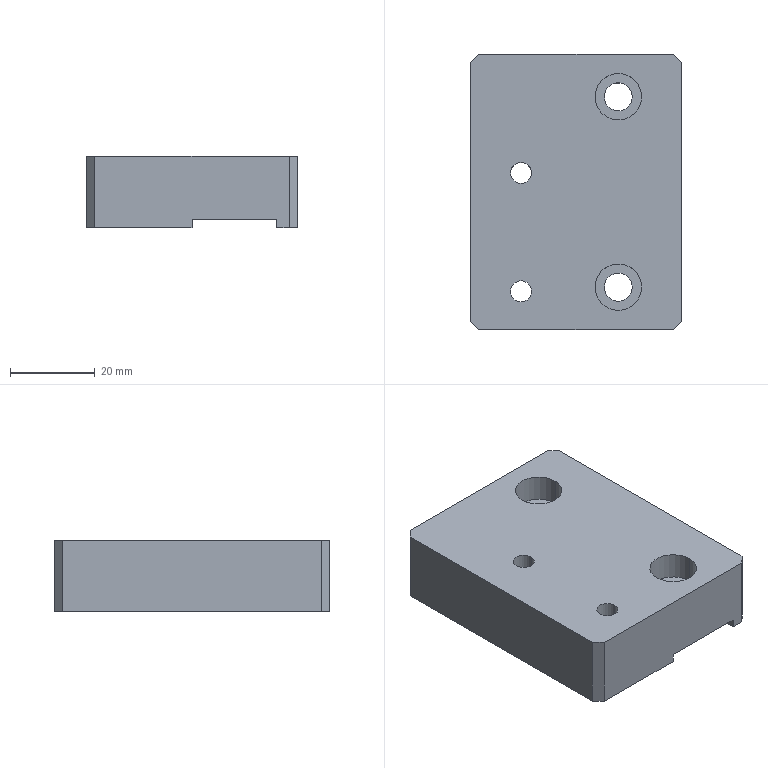Part | SolidWorks | features HoleWzd 2, Chamfer 1, Extrusion 1, ICE 1 | 1 solid | 28 faces | box 50 x 65 x 17 mm | volume 50042 mm3 | plane 16 | cylinder 12 | commonest cylinder face diameters 5 x4 6.6 x4 11 x4
STEP:
#1=CARTESIAN_POINT('',(29.5,-10.,10.6));
#2=VERTEX_POINT('',#1);
#3=CARTESIAN_POINT('',(40.5,-10.,10.6));
#4=VERTEX_POINT('',#3);
#5=CARTESIAN_POINT('',(35.,-10.,10.6));
#6=DIRECTION('',(0.,0.,1.));
#7=DIRECTION('',(1.,0.,0.));
#8=AXIS2_PLACEMENT_3D('',#5,#6,#7);
#9=CIRCLE('',#8,5.5);
#10=EDGE_CURVE('',#2,#4,#9,.T.);
#11=ORIENTED_EDGE('',*,*,#10,.F.);
#12=CARTESIAN_POINT('',(29.5,-10.,17.));
#13=VERTEX_POINT('',#12);
#14=CARTESIAN_POINT('',(29.5,-10.,17.));
#15=DIRECTION('',(0.,0.,1.));
#16=VECTOR('',#15,1000.);
#17=LINE('',#14,#16);
#18=EDGE_CURVE('',#2,#13,#17,.T.);
#19=ORIENTED_EDGE('',*,*,#18,.T.);
#20=CARTESIAN_POINT('',(40.5,-10.,17.));
#21=VERTEX_POINT('',#20);
#22=CARTESIAN_POINT('',(35.,-10.,17.));
#23=DIRECTION('',(0.,0.,1.));
#24=DIRECTION('',(1.,0.,0.));
#25=AXIS2_PLACEMENT_3D('',#22,#23,#24);
#26=CIRCLE('',#25,5.5);
#27=EDGE_CURVE('',#13,#21,#26,.T.);
#28=ORIENTED_EDGE('',*,*,#27,.T.);
#29=CARTESIAN_POINT('',(40.5,-10.,17.));
#30=DIRECTION('',(0.,0.,1.));
#31=VECTOR('',#30,1000.);
#32=LINE('',#29,#31);
#33=EDGE_CURVE('',#4,#21,#32,.T.);
#34=ORIENTED_EDGE('',*,*,#33,.F.);
#35=EDGE_LOOP('',(#11,#19,#28,#34));
#36=FACE_OUTER_BOUND('',#35,.T.);
#37=CARTESIAN_POINT('',(35.,-10.,17.));
#38=DIRECTION('',(0.,0.,1.));
#39=DIRECTION('',(1.,0.,0.));
#40=AXIS2_PLACEMENT_3D('',#37,#38,#39);
#41=CYLINDRICAL_SURFACE('',#40,5.5);
#42=ADVANCED_FACE('',(#36),#41,.F.);
#43=CARTESIAN_POINT('',(31.7,-10.,2.));
#44=VERTEX_POINT('',#43);
#45=CARTESIAN_POINT('',(38.3,-10.,2.));
#46=VERTEX_POINT('',#45);
#47=CARTESIAN_POINT('',(35.,-10.,2.));
#48=DIRECTION('',(0.,0.,1.));
#49=DIRECTION('',(1.,0.,0.));
#50=AXIS2_PLACEMENT_3D('',#47,#48,#49);
#51=CIRCLE('',#50,3.3);
#52=EDGE_CURVE('',#44,#46,#51,.T.);
#53=ORIENTED_EDGE('',*,*,#52,.F.);
#54=CARTESIAN_POINT('',(31.7,-10.,10.6));
#55=VERTEX_POINT('',#54);
#56=CARTESIAN_POINT('',(31.7,-10.,17.));
#57=DIRECTION('',(0.,0.,1.));
#58=VECTOR('',#57,1000.);
#59=LINE('',#56,#58);
#60=EDGE_CURVE('',#44,#55,#59,.T.);
#61=ORIENTED_EDGE('',*,*,#60,.T.);
#62=CARTESIAN_POINT('',(38.3,-10.,10.6));
#63=VERTEX_POINT('',#62);
#64=CARTESIAN_POINT('',(35.,-10.,10.6));
#65=DIRECTION('',(0.,0.,1.));
#66=DIRECTION('',(1.,0.,0.));
#67=AXIS2_PLACEMENT_3D('',#64,#65,#66);
#68=CIRCLE('',#67,3.3);
#69=EDGE_CURVE('',#55,#63,#68,.T.);
#70=ORIENTED_EDGE('',*,*,#69,.T.);
#71=CARTESIAN_POINT('',(38.3,-10.,17.));
#72=DIRECTION('',(0.,0.,1.));
#73=VECTOR('',#72,1000.);
#74=LINE('',#71,#73);
#75=EDGE_CURVE('',#46,#63,#74,.T.);
#76=ORIENTED_EDGE('',*,*,#75,.F.);
#77=EDGE_LOOP('',(#53,#61,#70,#76));
#78=FACE_OUTER_BOUND('',#77,.T.);
#79=CARTESIAN_POINT('',(35.,-10.,17.));
#80=DIRECTION('',(0.,0.,1.));
#81=DIRECTION('',(1.,0.,0.));
#82=AXIS2_PLACEMENT_3D('',#79,#80,#81);
#83=CYLINDRICAL_SURFACE('',#82,3.3);
#84=ADVANCED_FACE('',(#78),#83,.F.);
#85=CARTESIAN_POINT('',(29.5,-55.,10.6));
#86=VERTEX_POINT('',#85);
#87=CARTESIAN_POINT('',(40.5,-55.,10.6));
#88=VERTEX_POINT('',#87);
#89=CARTESIAN_POINT('',(35.,-55.,10.6));
#90=DIRECTION('',(0.,0.,1.));
#91=DIRECTION('',(1.,0.,0.));
#92=AXIS2_PLACEMENT_3D('',#89,#90,#91);
#93=CIRCLE('',#92,5.5);
#94=EDGE_CURVE('',#86,#88,#93,.T.);
#95=ORIENTED_EDGE('',*,*,#94,.F.);
#96=CARTESIAN_POINT('',(29.5,-55.,17.));
#97=VERTEX_POINT('',#96);
#98=CARTESIAN_POINT('',(29.5,-55.,17.));
#99=DIRECTION('',(0.,0.,1.));
#100=VECTOR('',#99,1000.);
#101=LINE('',#98,#100);
#102=EDGE_CURVE('',#86,#97,#101,.T.);
#103=ORIENTED_EDGE('',*,*,#102,.T.);
#104=CARTESIAN_POINT('',(40.5,-55.,17.));
#105=VERTEX_POINT('',#104);
#106=CARTESIAN_POINT('',(35.,-55.,17.));
#107=DIRECTION('',(0.,0.,1.));
#108=DIRECTION('',(1.,0.,0.));
#109=AXIS2_PLACEMENT_3D('',#106,#107,#108);
#110=CIRCLE('',#109,5.5);
#111=EDGE_CURVE('',#97,#105,#110,.T.);
#112=ORIENTED_EDGE('',*,*,#111,.T.);
#113=CARTESIAN_POINT('',(40.5,-55.,17.));
#114=DIRECTION('',(0.,0.,1.));
#115=VECTOR('',#114,1000.);
#116=LINE('',#113,#115);
#117=EDGE_CURVE('',#88,#105,#116,.T.);
#118=ORIENTED_EDGE('',*,*,#117,.F.);
#119=EDGE_LOOP('',(#95,#103,#112,#118));
#120=FACE_OUTER_BOUND('',#119,.T.);
#121=CARTESIAN_POINT('',(35.,-55.,17.));
#122=DIRECTION('',(0.,0.,1.));
#123=DIRECTION('',(1.,0.,0.));
#124=AXIS2_PLACEMENT_3D('',#121,#122,#123);
#125=CYLINDRICAL_SURFACE('',#124,5.5);
#126=ADVANCED_FACE('',(#120),#125,.F.);
#127=CARTESIAN_POINT('',(31.7,-55.,2.));
#128=VERTEX_POINT('',#127);
#129=CARTESIAN_POINT('',(38.3,-55.,2.));
#130=VERTEX_POINT('',#129);
#131=CARTESIAN_POINT('',(35.,-55.,2.));
#132=DIRECTION('',(0.,0.,1.));
#133=DIRECTION('',(1.,0.,0.));
#134=AXIS2_PLACEMENT_3D('',#131,#132,#133);
#135=CIRCLE('',#134,3.3);
#136=EDGE_CURVE('',#128,#130,#135,.T.);
#137=ORIENTED_EDGE('',*,*,#136,.F.);
#138=CARTESIAN_POINT('',(31.7,-55.,10.6));
#139=VERTEX_POINT('',#138);
#140=CARTESIAN_POINT('',(31.7,-55.,17.));
#141=DIRECTION('',(0.,0.,1.));
#142=VECTOR('',#141,1000.);
#143=LINE('',#140,#142);
#144=EDGE_CURVE('',#128,#139,#143,.T.);
#145=ORIENTED_EDGE('',*,*,#144,.T.);
#146=CARTESIAN_POINT('',(38.3,-55.,10.6));
#147=VERTEX_POINT('',#146);
#148=CARTESIAN_POINT('',(35.,-55.,10.6));
#149=DIRECTION('',(0.,0.,1.));
#150=DIRECTION('',(1.,0.,0.));
#151=AXIS2_PLACEMENT_3D('',#148,#149,#150);
#152=CIRCLE('',#151,3.3);
#153=EDGE_CURVE('',#139,#147,#152,.T.);
#154=ORIENTED_EDGE('',*,*,#153,.T.);
#155=CARTESIAN_POINT('',(38.3,-55.,17.));
#156=DIRECTION('',(0.,0.,1.));
#157=VECTOR('',#156,1000.);
#158=LINE('',#155,#157);
#159=EDGE_CURVE('',#130,#147,#158,.T.);
#160=ORIENTED_EDGE('',*,*,#159,.F.);
#161=EDGE_LOOP('',(#137,#145,#154,#160));
#162=FACE_OUTER_BOUND('',#161,.T.);
#163=CARTESIAN_POINT('',(35.,-55.,17.));
#164=DIRECTION('',(0.,0.,1.));
#165=DIRECTION('',(1.,0.,0.));
#166=AXIS2_PLACEMENT_3D('',#163,#164,#165);
#167=CYLINDRICAL_SURFACE('',#166,3.3);
#168=ADVANCED_FACE('',(#162),#167,.F.);
#169=CARTESIAN_POINT('',(9.5,-28.,0.));
#170=VERTEX_POINT('',#169);
#171=CARTESIAN_POINT('',(14.5,-28.,0.));
#172=VERTEX_POINT('',#171);
#173=CARTESIAN_POINT('',(12.,-28.,0.));
#174=DIRECTION('',(0.,0.,1.));
#175=DIRECTION('',(1.,0.,0.));
#176=AXIS2_PLACEMENT_3D('',#173,#174,#175);
#177=CIRCLE('',#176,2.5);
#178=EDGE_CURVE('',#170,#172,#177,.T.);
#179=ORIENTED_EDGE('',*,*,#178,.F.);
#180=CARTESIAN_POINT('',(9.5,-28.,17.));
#181=VERTEX_POINT('',#180);
#182=CARTESIAN_POINT('',(9.5,-28.,17.));
#183=DIRECTION('',(0.,0.,1.));
#184=VECTOR('',#183,1000.);
#185=LINE('',#182,#184);
#186=EDGE_CURVE('',#170,#181,#185,.T.);
#187=ORIENTED_EDGE('',*,*,#186,.T.);
#188=CARTESIAN_POINT('',(14.5,-28.,17.));
#189=VERTEX_POINT('',#188);
#190=CARTESIAN_POINT('',(12.,-28.,17.));
#191=DIRECTION('',(0.,0.,1.));
#192=DIRECTION('',(1.,0.,0.));
#193=AXIS2_PLACEMENT_3D('',#190,#191,#192);
#194=CIRCLE('',#193,2.5);
#195=EDGE_CURVE('',#181,#189,#194,.T.);
#196=ORIENTED_EDGE('',*,*,#195,.T.);
#197=CARTESIAN_POINT('',(14.5,-28.,17.));
#198=DIRECTION('',(0.,0.,1.));
#199=VECTOR('',#198,1000.);
#200=LINE('',#197,#199);
#201=EDGE_CURVE('',#172,#189,#200,.T.);
#202=ORIENTED_EDGE('',*,*,#201,.F.);
#203=EDGE_LOOP('',(#179,#187,#196,#202));
#204=FACE_OUTER_BOUND('',#203,.T.);
#205=CARTESIAN_POINT('',(12.,-28.,17.));
#206=DIRECTION('',(0.,0.,1.));
#207=DIRECTION('',(1.,0.,0.));
#208=AXIS2_PLACEMENT_3D('',#205,#206,#207);
#209=CYLINDRICAL_SURFACE('',#208,2.5);
#210=ADVANCED_FACE('',(#204),#209,.F.);
#211=CARTESIAN_POINT('',(9.5,-56.,0.));
#212=VERTEX_POINT('',#211);
#213=CARTESIAN_POINT('',(14.5,-56.,0.));
#214=VERTEX_POINT('',#213);
#215=CARTESIAN_POINT('',(12.,-56.,0.));
#216=DIRECTION('',(0.,0.,1.));
#217=DIRECTION('',(1.,0.,0.));
#218=AXIS2_PLACEMENT_3D('',#215,#216,#217);
#219=CIRCLE('',#218,2.5);
#220=EDGE_CURVE('',#212,#214,#219,.T.);
#221=ORIENTED_EDGE('',*,*,#220,.F.);
#222=CARTESIAN_POINT('',(9.5,-56.,17.));
#223=VERTEX_POINT('',#222);
#224=CARTESIAN_POINT('',(9.5,-56.,17.));
#225=DIRECTION('',(0.,0.,1.));
#226=VECTOR('',#225,1000.);
#227=LINE('',#224,#226);
#228=EDGE_CURVE('',#212,#223,#227,.T.);
#229=ORIENTED_EDGE('',*,*,#228,.T.);
#230=CARTESIAN_POINT('',(14.5,-56.,17.));
#231=VERTEX_POINT('',#230);
#232=CARTESIAN_POINT('',(12.,-56.,17.));
#233=DIRECTION('',(0.,0.,1.));
#234=DIRECTION('',(1.,0.,0.));
#235=AXIS2_PLACEMENT_3D('',#232,#233,#234);
#236=CIRCLE('',#235,2.5);
#237=EDGE_CURVE('',#223,#231,#236,.T.);
#238=ORIENTED_EDGE('',*,*,#237,.T.);
#239=CARTESIAN_POINT('',(14.5,-56.,17.));
#240=DIRECTION('',(0.,0.,1.));
#241=VECTOR('',#240,1000.);
#242=LINE('',#239,#241);
#243=EDGE_CURVE('',#214,#231,#242,.T.);
#244=ORIENTED_EDGE('',*,*,#243,.F.);
#245=EDGE_LOOP('',(#221,#229,#238,#244));
#246=FACE_OUTER_BOUND('',#245,.T.);
#247=CARTESIAN_POINT('',(12.,-56.,17.));
#248=DIRECTION('',(0.,0.,1.));
#249=DIRECTION('',(1.,0.,0.));
#250=AXIS2_PLACEMENT_3D('',#247,#248,#249);
#251=CYLINDRICAL_SURFACE('',#250,2.5);
#252=ADVANCED_FACE('',(#246),#251,.F.);
#253=CARTESIAN_POINT('',(50.,-63.,0.));
#254=VERTEX_POINT('',#253);
#255=CARTESIAN_POINT('',(50.,-2.,0.));
#256=VERTEX_POINT('',#255);
#257=CARTESIAN_POINT('',(50.,0.,0.));
#258=DIRECTION('',(0.,1.,0.));
#259=VECTOR('',#258,1000.);
#260=LINE('',#257,#259);
#261=EDGE_CURVE('',#254,#256,#260,.T.);
#262=ORIENTED_EDGE('',*,*,#261,.F.);
#263=CARTESIAN_POINT('',(48.,-65.,0.));
#264=VERTEX_POINT('',#263);
#265=CARTESIAN_POINT('',(50.,-63.,0.));
#266=DIRECTION('',(-0.7071,-0.7071,0.));
#267=VECTOR('',#266,1000.);
#268=LINE('',#265,#267);
#269=EDGE_CURVE('',#254,#264,#268,.T.);
#270=ORIENTED_EDGE('',*,*,#269,.T.);
#271=CARTESIAN_POINT('',(45.,-65.,0.));
#272=VERTEX_POINT('',#271);
#273=CARTESIAN_POINT('',(0.,-65.,0.));
#274=DIRECTION('',(1.,0.,0.));
#275=VECTOR('',#274,1000.);
#276=LINE('',#273,#275);
#277=EDGE_CURVE('',#272,#264,#276,.T.);
#278=ORIENTED_EDGE('',*,*,#277,.F.);
#279=CARTESIAN_POINT('',(45.,0.,0.));
#280=VERTEX_POINT('',#279);
#281=CARTESIAN_POINT('',(45.,0.,0.));
#282=DIRECTION('',(0.,-1.,0.));
#283=VECTOR('',#282,1000.);
#284=LINE('',#281,#283);
#285=EDGE_CURVE('',#280,#272,#284,.T.);
#286=ORIENTED_EDGE('',*,*,#285,.F.);
#287=CARTESIAN_POINT('',(48.,0.,0.));
#288=VERTEX_POINT('',#287);
#289=CARTESIAN_POINT('',(0.,0.,0.));
#290=DIRECTION('',(-1.,0.,0.));
#291=VECTOR('',#290,1000.);
#292=LINE('',#289,#291);
#293=EDGE_CURVE('',#288,#280,#292,.T.);
#294=ORIENTED_EDGE('',*,*,#293,.F.);
#295=CARTESIAN_POINT('',(48.,0.,0.));
#296=DIRECTION('',(0.7071,-0.7071,0.));
#297=VECTOR('',#296,1000.);
#298=LINE('',#295,#297);
#299=EDGE_CURVE('',#288,#256,#298,.T.);
#300=ORIENTED_EDGE('',*,*,#299,.T.);
#301=EDGE_LOOP('',(#262,#270,#278,#286,#294,#300));
#302=FACE_OUTER_BOUND('',#301,.T.);
#303=CARTESIAN_POINT('',(0.,0.,0.));
#304=DIRECTION('',(0.,0.,1.));
#305=DIRECTION('',(1.,0.,0.));
#306=AXIS2_PLACEMENT_3D('',#303,#304,#305);
#307=PLANE('',#306);
#308=ADVANCED_FACE('',(#302),#307,.F.);
#309=CARTESIAN_POINT('',(0.,-2.,17.));
#310=VERTEX_POINT('',#309);
#311=CARTESIAN_POINT('',(0.,-63.,17.));
#312=VERTEX_POINT('',#311);
#313=CARTESIAN_POINT('',(0.,0.,17.));
#314=DIRECTION('',(0.,-1.,0.));
#315=VECTOR('',#314,1000.);
#316=LINE('',#313,#315);
#317=EDGE_CURVE('',#310,#312,#316,.T.);
#318=ORIENTED_EDGE('',*,*,#317,.F.);
#319=CARTESIAN_POINT('',(0.,-2.,0.));
#320=VERTEX_POINT('',#319);
#321=CARTESIAN_POINT('',(0.,-2.,17.));
#322=DIRECTION('',(0.,0.,-1.));
#323=VECTOR('',#322,1000.);
#324=LINE('',#321,#323);
#325=EDGE_CURVE('',#310,#320,#324,.T.);
#326=ORIENTED_EDGE('',*,*,#325,.T.);
#327=CARTESIAN_POINT('',(0.,-63.,0.));
#328=VERTEX_POINT('',#327);
#329=CARTESIAN_POINT('',(0.,0.,0.));
#330=DIRECTION('',(0.,-1.,0.));
#331=VECTOR('',#330,1000.);
#332=LINE('',#329,#331);
#333=EDGE_CURVE('',#320,#328,#332,.T.);
#334=ORIENTED_EDGE('',*,*,#333,.T.);
#335=CARTESIAN_POINT('',(0.,-63.,17.));
#336=DIRECTION('',(0.,0.,1.));
#337=VECTOR('',#336,1000.);
#338=LINE('',#335,#337);
#339=EDGE_CURVE('',#328,#312,#338,.T.);
#340=ORIENTED_EDGE('',*,*,#339,.T.);
#341=EDGE_LOOP('',(#318,#326,#334,#340));
#342=FACE_OUTER_BOUND('',#341,.T.);
#343=CARTESIAN_POINT('',(0.,0.,17.));
#344=DIRECTION('',(1.,0.,0.));
#345=DIRECTION('',(0.,0.,-1.));
#346=AXIS2_PLACEMENT_3D('',#343,#344,#345);
#347=PLANE('',#346);
#348=ADVANCED_FACE('',(#342),#347,.F.);
#349=ORIENTED_EDGE('',*,*,#277,.T.);
#350=CARTESIAN_POINT('',(48.,-65.,17.));
#351=VERTEX_POINT('',#350);
#352=CARTESIAN_POINT('',(48.,-65.,17.));
#353=DIRECTION('',(0.,0.,1.));
#354=VECTOR('',#353,1000.);
#355=LINE('',#352,#354);
#356=EDGE_CURVE('',#264,#351,#355,.T.);
#357=ORIENTED_EDGE('',*,*,#356,.T.);
#358=CARTESIAN_POINT('',(2.,-65.,17.));
#359=VERTEX_POINT('',#358);
#360=CARTESIAN_POINT('',(0.,-65.,17.));
#361=DIRECTION('',(1.,0.,0.));
#362=VECTOR('',#361,1000.);
#363=LINE('',#360,#362);
#364=EDGE_CURVE('',#359,#351,#363,.T.);
#365=ORIENTED_EDGE('',*,*,#364,.F.);
#366=CARTESIAN_POINT('',(2.,-65.,0.));
#367=VERTEX_POINT('',#366);
#368=CARTESIAN_POINT('',(2.,-65.,17.));
#369=DIRECTION('',(0.,0.,-1.));
#370=VECTOR('',#369,1000.);
#371=LINE('',#368,#370);
#372=EDGE_CURVE('',#359,#367,#371,.T.);
#373=ORIENTED_EDGE('',*,*,#372,.T.);
#374=CARTESIAN_POINT('',(25.,-65.,0.));
#375=VERTEX_POINT('',#374);
#376=CARTESIAN_POINT('',(0.,-65.,0.));
#377=DIRECTION('',(1.,0.,0.));
#378=VECTOR('',#377,1000.);
#379=LINE('',#376,#378);
#380=EDGE_CURVE('',#367,#375,#379,.T.);
#381=ORIENTED_EDGE('',*,*,#380,.T.);
#382=CARTESIAN_POINT('',(25.,-65.,2.));
#383=VERTEX_POINT('',#382);
#384=CARTESIAN_POINT('',(25.,-65.,0.));
#385=DIRECTION('',(0.,0.,-1.));
#386=VECTOR('',#385,1000.);
#387=LINE('',#384,#386);
#388=EDGE_CURVE('',#383,#375,#387,.T.);
#389=ORIENTED_EDGE('',*,*,#388,.F.);
#390=CARTESIAN_POINT('',(45.,-65.,2.));
#391=VERTEX_POINT('',#390);
#392=CARTESIAN_POINT('',(45.,-65.,2.));
#393=DIRECTION('',(-1.,0.,0.));
#394=VECTOR('',#393,1000.);
#395=LINE('',#392,#394);
#396=EDGE_CURVE('',#391,#383,#395,.T.);
#397=ORIENTED_EDGE('',*,*,#396,.F.);
#398=CARTESIAN_POINT('',(45.,-65.,0.));
#399=DIRECTION('',(0.,0.,1.));
#400=VECTOR('',#399,1000.);
#401=LINE('',#398,#400);
#402=EDGE_CURVE('',#272,#391,#401,.T.);
#403=ORIENTED_EDGE('',*,*,#402,.F.);
#404=EDGE_LOOP('',(#349,#357,#365,#373,#381,#389,#397,#403));
#405=FACE_OUTER_BOUND('',#404,.T.);
#406=CARTESIAN_POINT('',(0.,-65.,17.));
#407=DIRECTION('',(0.,1.,0.));
#408=DIRECTION('',(0.,0.,1.));
#409=AXIS2_PLACEMENT_3D('',#406,#407,#408);
#410=PLANE('',#409);
#411=ADVANCED_FACE('',(#405),#410,.F.);
#412=CARTESIAN_POINT('',(50.,-63.,17.));
#413=VERTEX_POINT('',#412);
#414=CARTESIAN_POINT('',(50.,-2.,17.));
#415=VERTEX_POINT('',#414);
#416=CARTESIAN_POINT('',(50.,0.,17.));
#417=DIRECTION('',(0.,1.,0.));
#418=VECTOR('',#417,1000.);
#419=LINE('',#416,#418);
#420=EDGE_CURVE('',#413,#415,#419,.T.);
#421=ORIENTED_EDGE('',*,*,#420,.F.);
#422=CARTESIAN_POINT('',(50.,-63.,17.));
#423=DIRECTION('',(0.,0.,-1.));
#424=VECTOR('',#423,1000.);
#425=LINE('',#422,#424);
#426=EDGE_CURVE('',#413,#254,#425,.T.);
#427=ORIENTED_EDGE('',*,*,#426,.T.);
#428=ORIENTED_EDGE('',*,*,#261,.T.);
#429=CARTESIAN_POINT('',(50.,-2.,17.));
#430=DIRECTION('',(0.,0.,1.));
#431=VECTOR('',#430,1000.);
#432=LINE('',#429,#431);
#433=EDGE_CURVE('',#256,#415,#432,.T.);
#434=ORIENTED_EDGE('',*,*,#433,.T.);
#435=EDGE_LOOP('',(#421,#427,#428,#434));
#436=FACE_OUTER_BOUND('',#435,.T.);
#437=CARTESIAN_POINT('',(50.,0.,17.));
#438=DIRECTION('',(-1.,0.,0.));
#439=DIRECTION('',(0.,-1.,0.));
#440=AXIS2_PLACEMENT_3D('',#437,#438,#439);
#441=PLANE('',#440);
#442=ADVANCED_FACE('',(#436),#441,.F.);
#443=CARTESIAN_POINT('',(48.,0.,17.));
#444=VERTEX_POINT('',#443);
#445=CARTESIAN_POINT('',(2.,0.,17.));
#446=VERTEX_POINT('',#445);
#447=CARTESIAN_POINT('',(0.,0.,17.));
#448=DIRECTION('',(-1.,0.,0.));
#449=VECTOR('',#448,1000.);
#450=LINE('',#447,#449);
#451=EDGE_CURVE('',#444,#446,#450,.T.);
#452=ORIENTED_EDGE('',*,*,#451,.F.);
#453=CARTESIAN_POINT('',(48.,0.,17.));
#454=DIRECTION('',(0.,0.,-1.));
#455=VECTOR('',#454,1000.);
#456=LINE('',#453,#455);
#457=EDGE_CURVE('',#444,#288,#456,.T.);
#458=ORIENTED_EDGE('',*,*,#457,.T.);
#459=ORIENTED_EDGE('',*,*,#293,.T.);
#460=CARTESIAN_POINT('',(45.,0.,2.));
#461=VERTEX_POINT('',#460);
#462=CARTESIAN_POINT('',(45.,0.,0.));
#463=DIRECTION('',(0.,0.,1.));
#464=VECTOR('',#463,1000.);
#465=LINE('',#462,#464);
#466=EDGE_CURVE('',#280,#461,#465,.T.);
#467=ORIENTED_EDGE('',*,*,#466,.T.);
#468=CARTESIAN_POINT('',(25.,0.,2.));
#469=VERTEX_POINT('',#468);
#470=CARTESIAN_POINT('',(45.,0.,2.));
#471=DIRECTION('',(-1.,0.,0.));
#472=VECTOR('',#471,1000.);
#473=LINE('',#470,#472);
#474=EDGE_CURVE('',#461,#469,#473,.T.);
#475=ORIENTED_EDGE('',*,*,#474,.T.);
#476=CARTESIAN_POINT('',(25.,0.,0.));
#477=VERTEX_POINT('',#476);
#478=CARTESIAN_POINT('',(25.,0.,0.));
#479=DIRECTION('',(0.,0.,-1.));
#480=VECTOR('',#479,1000.);
#481=LINE('',#478,#480);
#482=EDGE_CURVE('',#469,#477,#481,.T.);
#483=ORIENTED_EDGE('',*,*,#482,.T.);
#484=CARTESIAN_POINT('',(2.,0.,0.));
#485=VERTEX_POINT('',#484);
#486=CARTESIAN_POINT('',(0.,0.,0.));
#487=DIRECTION('',(-1.,0.,0.));
#488=VECTOR('',#487,1000.);
#489=LINE('',#486,#488);
#490=EDGE_CURVE('',#477,#485,#489,.T.);
#491=ORIENTED_EDGE('',*,*,#490,.T.);
#492=CARTESIAN_POINT('',(2.,0.,17.));
#493=DIRECTION('',(0.,0.,1.));
#494=VECTOR('',#493,1000.);
#495=LINE('',#492,#494);
#496=EDGE_CURVE('',#485,#446,#495,.T.);
#497=ORIENTED_EDGE('',*,*,#496,.T.);
#498=EDGE_LOOP('',(#452,#458,#459,#467,#475,#483,#491,#497));
#499=FACE_OUTER_BOUND('',#498,.T.);
#500=CARTESIAN_POINT('',(0.,0.,17.));
#501=DIRECTION('',(0.,-1.,0.));
#502=DIRECTION('',(0.,0.,-1.));
#503=AXIS2_PLACEMENT_3D('',#500,#501,#502);
#504=PLANE('',#503);
#505=ADVANCED_FACE('',(#499),#504,.F.);
#506=CARTESIAN_POINT('',(35.,-10.,17.));
#507=DIRECTION('',(0.,0.,1.));
#508=DIRECTION('',(1.,0.,0.));
#509=AXIS2_PLACEMENT_3D('',#506,#507,#508);
#510=CIRCLE('',#509,5.5);
#511=EDGE_CURVE('',#21,#13,#510,.T.);
#512=ORIENTED_EDGE('',*,*,#511,.F.);
#513=ORIENTED_EDGE('',*,*,#27,.F.);
#514=EDGE_LOOP('',(#512,#513));
#515=FACE_BOUND('',#514,.T.);
#516=CARTESIAN_POINT('',(35.,-55.,17.));
#517=DIRECTION('',(0.,0.,1.));
#518=DIRECTION('',(1.,0.,0.));
#519=AXIS2_PLACEMENT_3D('',#516,#517,#518);
#520=CIRCLE('',#519,5.5);
#521=EDGE_CURVE('',#105,#97,#520,.T.);
#522=ORIENTED_EDGE('',*,*,#521,.F.);
#523=ORIENTED_EDGE('',*,*,#111,.F.);
#524=EDGE_LOOP('',(#522,#523));
#525=FACE_BOUND('',#524,.T.);
#526=CARTESIAN_POINT('',(12.,-28.,17.));
#527=DIRECTION('',(0.,0.,1.));
#528=DIRECTION('',(1.,0.,0.));
#529=AXIS2_PLACEMENT_3D('',#526,#527,#528);
#530=CIRCLE('',#529,2.5);
#531=EDGE_CURVE('',#189,#181,#530,.T.);
#532=ORIENTED_EDGE('',*,*,#531,.F.);
#533=ORIENTED_EDGE('',*,*,#195,.F.);
#534=EDGE_LOOP('',(#532,#533));
#535=FACE_BOUND('',#534,.T.);
#536=CARTESIAN_POINT('',(12.,-56.,17.));
#537=DIRECTION('',(0.,0.,1.));
#538=DIRECTION('',(1.,0.,0.));
#539=AXIS2_PLACEMENT_3D('',#536,#537,#538);
#540=CIRCLE('',#539,2.5);
#541=EDGE_CURVE('',#231,#223,#540,.T.);
#542=ORIENTED_EDGE('',*,*,#541,.F.);
#543=ORIENTED_EDGE('',*,*,#237,.F.);
#544=EDGE_LOOP('',(#542,#543));
#545=FACE_BOUND('',#544,.T.);
#546=ORIENTED_EDGE('',*,*,#364,.T.);
#547=CARTESIAN_POINT('',(56.5,-56.5,17.));
#548=DIRECTION('',(0.7071,0.7071,0.));
#549=VECTOR('',#548,1000.);
#550=LINE('',#547,#549);
#551=EDGE_CURVE('',#351,#413,#550,.T.);
#552=ORIENTED_EDGE('',*,*,#551,.T.);
#553=ORIENTED_EDGE('',*,*,#420,.T.);
#554=CARTESIAN_POINT('',(24.,24.,17.));
#555=DIRECTION('',(-0.7071,0.7071,0.));
#556=VECTOR('',#555,1000.);
#557=LINE('',#554,#556);
#558=EDGE_CURVE('',#415,#444,#557,.T.);
#559=ORIENTED_EDGE('',*,*,#558,.T.);
#560=ORIENTED_EDGE('',*,*,#451,.T.);
#561=CARTESIAN_POINT('',(1.,-1.,17.));
#562=DIRECTION('',(-0.7071,-0.7071,0.));
#563=VECTOR('',#562,1000.);
#564=LINE('',#561,#563);
#565=EDGE_CURVE('',#446,#310,#564,.T.);
#566=ORIENTED_EDGE('',*,*,#565,.T.);
#567=ORIENTED_EDGE('',*,*,#317,.T.);
#568=CARTESIAN_POINT('',(-31.5,-31.5,17.));
#569=DIRECTION('',(0.7071,-0.7071,0.));
#570=VECTOR('',#569,1000.);
#571=LINE('',#568,#570);
#572=EDGE_CURVE('',#312,#359,#571,.T.);
#573=ORIENTED_EDGE('',*,*,#572,.T.);
#574=EDGE_LOOP('',(#546,#552,#553,#559,#560,#566,#567,#573));
#575=FACE_OUTER_BOUND('',#574,.T.);
#576=CARTESIAN_POINT('',(0.,0.,17.));
#577=DIRECTION('',(0.,0.,1.));
#578=DIRECTION('',(1.,0.,0.));
#579=AXIS2_PLACEMENT_3D('',#576,#577,#578);
#580=PLANE('',#579);
#581=ADVANCED_FACE('',(#515,#525,#535,#545,#575),#580,.T.);
#582=CARTESIAN_POINT('',(12.,-28.,0.));
#583=DIRECTION('',(0.,0.,1.));
#584=DIRECTION('',(1.,0.,0.));
#585=AXIS2_PLACEMENT_3D('',#582,#583,#584);
#586=CIRCLE('',#585,2.5);
#587=EDGE_CURVE('',#172,#170,#586,.T.);
#588=ORIENTED_EDGE('',*,*,#587,.T.);
#589=ORIENTED_EDGE('',*,*,#178,.T.);
#590=EDGE_LOOP('',(#588,#589));
#591=FACE_BOUND('',#590,.T.);
#592=CARTESIAN_POINT('',(12.,-56.,0.));
#593=DIRECTION('',(0.,0.,1.));
#594=DIRECTION('',(1.,0.,0.));
#595=AXIS2_PLACEMENT_3D('',#592,#593,#594);
#596=CIRCLE('',#595,2.5);
#597=EDGE_CURVE('',#214,#212,#596,.T.);
#598=ORIENTED_EDGE('',*,*,#597,.T.);
#599=ORIENTED_EDGE('',*,*,#220,.T.);
#600=EDGE_LOOP('',(#598,#599));
#601=FACE_BOUND('',#600,.T.);
#602=ORIENTED_EDGE('',*,*,#333,.F.);
#603=CARTESIAN_POINT('',(0.,-2.,0.));
#604=DIRECTION('',(0.7071,0.7071,0.));
#605=VECTOR('',#604,1000.);
#606=LINE('',#603,#605);
#607=EDGE_CURVE('',#320,#485,#606,.T.);
#608=ORIENTED_EDGE('',*,*,#607,.T.);
#609=ORIENTED_EDGE('',*,*,#490,.F.);
#610=CARTESIAN_POINT('',(25.,0.,0.));
#611=DIRECTION('',(0.,-1.,0.));
#612=VECTOR('',#611,1000.);
#613=LINE('',#610,#612);
#614=EDGE_CURVE('',#477,#375,#613,.T.);
#615=ORIENTED_EDGE('',*,*,#614,.T.);
#616=ORIENTED_EDGE('',*,*,#380,.F.);
#617=CARTESIAN_POINT('',(2.,-65.,0.));
#618=DIRECTION('',(-0.7071,0.7071,0.));
#619=VECTOR('',#618,1000.);
#620=LINE('',#617,#619);
#621=EDGE_CURVE('',#367,#328,#620,.T.);
#622=ORIENTED_EDGE('',*,*,#621,.T.);
#623=EDGE_LOOP('',(#602,#608,#609,#615,#616,#622));
#624=FACE_OUTER_BOUND('',#623,.T.);
#625=CARTESIAN_POINT('',(0.,0.,0.));
#626=DIRECTION('',(0.,0.,1.));
#627=DIRECTION('',(1.,0.,0.));
#628=AXIS2_PLACEMENT_3D('',#625,#626,#627);
#629=PLANE('',#628);
#630=ADVANCED_FACE('',(#591,#601,#624),#629,.F.);
#631=ORIENTED_EDGE('',*,*,#402,.T.);
#632=CARTESIAN_POINT('',(45.,0.,2.));
#633=DIRECTION('',(0.,-1.,0.));
#634=VECTOR('',#633,1000.);
#635=LINE('',#632,#634);
#636=EDGE_CURVE('',#461,#391,#635,.T.);
#637=ORIENTED_EDGE('',*,*,#636,.F.);
#638=ORIENTED_EDGE('',*,*,#466,.F.);
#639=ORIENTED_EDGE('',*,*,#285,.T.);
#640=EDGE_LOOP('',(#631,#637,#638,#639));
#641=FACE_OUTER_BOUND('',#640,.T.);
#642=CARTESIAN_POINT('',(45.,0.,0.));
#643=DIRECTION('',(1.,0.,0.));
#644=DIRECTION('',(0.,0.,-1.));
#645=AXIS2_PLACEMENT_3D('',#642,#643,#644);
#646=PLANE('',#645);
#647=ADVANCED_FACE('',(#641),#646,.F.);
#648=ORIENTED_EDGE('',*,*,#388,.T.);
#649=ORIENTED_EDGE('',*,*,#614,.F.);
#650=ORIENTED_EDGE('',*,*,#482,.F.);
#651=CARTESIAN_POINT('',(25.,0.,2.));
#652=DIRECTION('',(0.,-1.,0.));
#653=VECTOR('',#652,1000.);
#654=LINE('',#651,#653);
#655=EDGE_CURVE('',#469,#383,#654,.T.);
#656=ORIENTED_EDGE('',*,*,#655,.T.);
#657=EDGE_LOOP('',(#648,#649,#650,#656));
#658=FACE_OUTER_BOUND('',#657,.T.);
#659=CARTESIAN_POINT('',(25.,0.,0.));
#660=DIRECTION('',(-1.,0.,0.));
#661=DIRECTION('',(0.,0.,1.));
#662=AXIS2_PLACEMENT_3D('',#659,#660,#661);
#663=PLANE('',#662);
#664=ADVANCED_FACE('',(#658),#663,.F.);
#665=CARTESIAN_POINT('',(35.,-10.,2.));
#666=DIRECTION('',(0.,0.,1.));
#667=DIRECTION('',(1.,0.,0.));
#668=AXIS2_PLACEMENT_3D('',#665,#666,#667);
#669=CIRCLE('',#668,3.3);
#670=EDGE_CURVE('',#46,#44,#669,.T.);
#671=ORIENTED_EDGE('',*,*,#670,.T.);
#672=ORIENTED_EDGE('',*,*,#52,.T.);
#673=EDGE_LOOP('',(#671,#672));
#674=FACE_BOUND('',#673,.T.);
#675=CARTESIAN_POINT('',(35.,-55.,2.));
#676=DIRECTION('',(0.,0.,1.));
#677=DIRECTION('',(1.,0.,0.));
#678=AXIS2_PLACEMENT_3D('',#675,#676,#677);
#679=CIRCLE('',#678,3.3);
#680=EDGE_CURVE('',#130,#128,#679,.T.);
#681=ORIENTED_EDGE('',*,*,#680,.T.);
#682=ORIENTED_EDGE('',*,*,#136,.T.);
#683=EDGE_LOOP('',(#681,#682));
#684=FACE_BOUND('',#683,.T.);
#685=ORIENTED_EDGE('',*,*,#396,.T.);
#686=ORIENTED_EDGE('',*,*,#655,.F.);
#687=ORIENTED_EDGE('',*,*,#474,.F.);
#688=ORIENTED_EDGE('',*,*,#636,.T.);
#689=EDGE_LOOP('',(#685,#686,#687,#688));
#690=FACE_OUTER_BOUND('',#689,.T.);
#691=CARTESIAN_POINT('',(45.,0.,2.));
#692=DIRECTION('',(0.,0.,1.));
#693=DIRECTION('',(1.,0.,0.));
#694=AXIS2_PLACEMENT_3D('',#691,#692,#693);
#695=PLANE('',#694);
#696=ADVANCED_FACE('',(#674,#684,#690),#695,.F.);
#697=ORIENTED_EDGE('',*,*,#551,.F.);
#698=ORIENTED_EDGE('',*,*,#356,.F.);
#699=ORIENTED_EDGE('',*,*,#269,.F.);
#700=ORIENTED_EDGE('',*,*,#426,.F.);
#701=EDGE_LOOP('',(#697,#698,#699,#700));
#702=FACE_OUTER_BOUND('',#701,.T.);
#703=CARTESIAN_POINT('',(50.,-63.,17.));
#704=DIRECTION('',(-0.7071,0.7071,0.));
#705=DIRECTION('',(0.,0.,-1.));
#706=AXIS2_PLACEMENT_3D('',#703,#704,#705);
#707=PLANE('',#706);
#708=ADVANCED_FACE('',(#702),#707,.F.);
#709=ORIENTED_EDGE('',*,*,#558,.F.);
#710=ORIENTED_EDGE('',*,*,#433,.F.);
#711=ORIENTED_EDGE('',*,*,#299,.F.);
#712=ORIENTED_EDGE('',*,*,#457,.F.);
#713=EDGE_LOOP('',(#709,#710,#711,#712));
#714=FACE_OUTER_BOUND('',#713,.T.);
#715=CARTESIAN_POINT('',(48.,0.,17.));
#716=DIRECTION('',(-0.7071,-0.7071,0.));
#717=DIRECTION('',(0.,0.,-1.));
#718=AXIS2_PLACEMENT_3D('',#715,#716,#717);
#719=PLANE('',#718);
#720=ADVANCED_FACE('',(#714),#719,.F.);
#721=ORIENTED_EDGE('',*,*,#565,.F.);
#722=ORIENTED_EDGE('',*,*,#496,.F.);
#723=ORIENTED_EDGE('',*,*,#607,.F.);
#724=ORIENTED_EDGE('',*,*,#325,.F.);
#725=EDGE_LOOP('',(#721,#722,#723,#724));
#726=FACE_OUTER_BOUND('',#725,.T.);
#727=CARTESIAN_POINT('',(0.,-2.,17.));
#728=DIRECTION('',(0.7071,-0.7071,0.));
#729=DIRECTION('',(0.,0.,-1.));
#730=AXIS2_PLACEMENT_3D('',#727,#728,#729);
#731=PLANE('',#730);
#732=ADVANCED_FACE('',(#726),#731,.F.);
#733=ORIENTED_EDGE('',*,*,#572,.F.);
#734=ORIENTED_EDGE('',*,*,#339,.F.);
#735=ORIENTED_EDGE('',*,*,#621,.F.);
#736=ORIENTED_EDGE('',*,*,#372,.F.);
#737=EDGE_LOOP('',(#733,#734,#735,#736));
#738=FACE_OUTER_BOUND('',#737,.T.);
#739=CARTESIAN_POINT('',(2.,-65.,17.));
#740=DIRECTION('',(0.7071,0.7071,0.));
#741=DIRECTION('',(0.,0.,-1.));
#742=AXIS2_PLACEMENT_3D('',#739,#740,#741);
#743=PLANE('',#742);
#744=ADVANCED_FACE('',(#738),#743,.F.);
#745=ORIENTED_EDGE('',*,*,#228,.F.);
#746=ORIENTED_EDGE('',*,*,#597,.F.);
#747=ORIENTED_EDGE('',*,*,#243,.T.);
#748=ORIENTED_EDGE('',*,*,#541,.T.);
#749=EDGE_LOOP('',(#745,#746,#747,#748));
#750=FACE_OUTER_BOUND('',#749,.T.);
#751=CARTESIAN_POINT('',(12.,-56.,17.));
#752=DIRECTION('',(0.,0.,1.));
#753=DIRECTION('',(1.,0.,0.));
#754=AXIS2_PLACEMENT_3D('',#751,#752,#753);
#755=CYLINDRICAL_SURFACE('',#754,2.5);
#756=ADVANCED_FACE('',(#750),#755,.F.);
#757=ORIENTED_EDGE('',*,*,#186,.F.);
#758=ORIENTED_EDGE('',*,*,#587,.F.);
#759=ORIENTED_EDGE('',*,*,#201,.T.);
#760=ORIENTED_EDGE('',*,*,#531,.T.);
#761=EDGE_LOOP('',(#757,#758,#759,#760));
#762=FACE_OUTER_BOUND('',#761,.T.);
#763=CARTESIAN_POINT('',(12.,-28.,17.));
#764=DIRECTION('',(0.,0.,1.));
#765=DIRECTION('',(1.,0.,0.));
#766=AXIS2_PLACEMENT_3D('',#763,#764,#765);
#767=CYLINDRICAL_SURFACE('',#766,2.5);
#768=ADVANCED_FACE('',(#762),#767,.F.);
#769=ORIENTED_EDGE('',*,*,#144,.F.);
#770=ORIENTED_EDGE('',*,*,#680,.F.);
#771=ORIENTED_EDGE('',*,*,#159,.T.);
#772=CARTESIAN_POINT('',(35.,-55.,10.6));
#773=DIRECTION('',(0.,0.,1.));
#774=DIRECTION('',(1.,0.,0.));
#775=AXIS2_PLACEMENT_3D('',#772,#773,#774);
#776=CIRCLE('',#775,3.3);
#777=EDGE_CURVE('',#147,#139,#776,.T.);
#778=ORIENTED_EDGE('',*,*,#777,.T.);
#779=EDGE_LOOP('',(#769,#770,#771,#778));
#780=FACE_OUTER_BOUND('',#779,.T.);
#781=CARTESIAN_POINT('',(35.,-55.,17.));
#782=DIRECTION('',(0.,0.,1.));
#783=DIRECTION('',(1.,0.,0.));
#784=AXIS2_PLACEMENT_3D('',#781,#782,#783);
#785=CYLINDRICAL_SURFACE('',#784,3.3);
#786=ADVANCED_FACE('',(#780),#785,.F.);
#787=ORIENTED_EDGE('',*,*,#777,.F.);
#788=ORIENTED_EDGE('',*,*,#153,.F.);
#789=EDGE_LOOP('',(#787,#788));
#790=FACE_BOUND('',#789,.T.);
#791=CARTESIAN_POINT('',(35.,-55.,10.6));
#792=DIRECTION('',(0.,0.,1.));
#793=DIRECTION('',(1.,0.,0.));
#794=AXIS2_PLACEMENT_3D('',#791,#792,#793);
#795=CIRCLE('',#794,5.5);
#796=EDGE_CURVE('',#88,#86,#795,.T.);
#797=ORIENTED_EDGE('',*,*,#796,.T.);
#798=ORIENTED_EDGE('',*,*,#94,.T.);
#799=EDGE_LOOP('',(#797,#798));
#800=FACE_OUTER_BOUND('',#799,.T.);
#801=CARTESIAN_POINT('',(38.3,-55.,10.6));
#802=DIRECTION('',(0.,0.,-1.));
#803=DIRECTION('',(-1.,0.,0.));
#804=AXIS2_PLACEMENT_3D('',#801,#802,#803);
#805=PLANE('',#804);
#806=ADVANCED_FACE('',(#790,#800),#805,.F.);
#807=ORIENTED_EDGE('',*,*,#102,.F.);
#808=ORIENTED_EDGE('',*,*,#796,.F.);
#809=ORIENTED_EDGE('',*,*,#117,.T.);
#810=ORIENTED_EDGE('',*,*,#521,.T.);
#811=EDGE_LOOP('',(#807,#808,#809,#810));
#812=FACE_OUTER_BOUND('',#811,.T.);
#813=CARTESIAN_POINT('',(35.,-55.,17.));
#814=DIRECTION('',(0.,0.,1.));
#815=DIRECTION('',(1.,0.,0.));
#816=AXIS2_PLACEMENT_3D('',#813,#814,#815);
#817=CYLINDRICAL_SURFACE('',#816,5.5);
#818=ADVANCED_FACE('',(#812),#817,.F.);
#819=ORIENTED_EDGE('',*,*,#60,.F.);
#820=ORIENTED_EDGE('',*,*,#670,.F.);
#821=ORIENTED_EDGE('',*,*,#75,.T.);
#822=CARTESIAN_POINT('',(35.,-10.,10.6));
#823=DIRECTION('',(0.,0.,1.));
#824=DIRECTION('',(1.,0.,0.));
#825=AXIS2_PLACEMENT_3D('',#822,#823,#824);
#826=CIRCLE('',#825,3.3);
#827=EDGE_CURVE('',#63,#55,#826,.T.);
#828=ORIENTED_EDGE('',*,*,#827,.T.);
#829=EDGE_LOOP('',(#819,#820,#821,#828));
#830=FACE_OUTER_BOUND('',#829,.T.);
#831=CARTESIAN_POINT('',(35.,-10.,17.));
#832=DIRECTION('',(0.,0.,1.));
#833=DIRECTION('',(1.,0.,0.));
#834=AXIS2_PLACEMENT_3D('',#831,#832,#833);
#835=CYLINDRICAL_SURFACE('',#834,3.3);
#836=ADVANCED_FACE('',(#830),#835,.F.);
#837=ORIENTED_EDGE('',*,*,#827,.F.);
#838=ORIENTED_EDGE('',*,*,#69,.F.);
#839=EDGE_LOOP('',(#837,#838));
#840=FACE_BOUND('',#839,.T.);
#841=CARTESIAN_POINT('',(35.,-10.,10.6));
#842=DIRECTION('',(0.,0.,1.));
#843=DIRECTION('',(1.,0.,0.));
#844=AXIS2_PLACEMENT_3D('',#841,#842,#843);
#845=CIRCLE('',#844,5.5);
#846=EDGE_CURVE('',#4,#2,#845,.T.);
#847=ORIENTED_EDGE('',*,*,#846,.T.);
#848=ORIENTED_EDGE('',*,*,#10,.T.);
#849=EDGE_LOOP('',(#847,#848));
#850=FACE_OUTER_BOUND('',#849,.T.);
#851=CARTESIAN_POINT('',(38.3,-10.,10.6));
#852=DIRECTION('',(0.,0.,-1.));
#853=DIRECTION('',(-1.,0.,0.));
#854=AXIS2_PLACEMENT_3D('',#851,#852,#853);
#855=PLANE('',#854);
#856=ADVANCED_FACE('',(#840,#850),#855,.F.);
#857=ORIENTED_EDGE('',*,*,#18,.F.);
#858=ORIENTED_EDGE('',*,*,#846,.F.);
#859=ORIENTED_EDGE('',*,*,#33,.T.);
#860=ORIENTED_EDGE('',*,*,#511,.T.);
#861=EDGE_LOOP('',(#857,#858,#859,#860));
#862=FACE_OUTER_BOUND('',#861,.T.);
#863=CARTESIAN_POINT('',(35.,-10.,17.));
#864=DIRECTION('',(0.,0.,1.));
#865=DIRECTION('',(1.,0.,0.));
#866=AXIS2_PLACEMENT_3D('',#863,#864,#865);
#867=CYLINDRICAL_SURFACE('',#866,5.5);
#868=ADVANCED_FACE('',(#862),#867,.F.);
#869=CLOSED_SHELL('',(#42,#84,#126,#168,#210,#252,#308,#348,#411,#442,#505,#581,#630,#647,#664,#696,#708,#720,#732,#744,#756,#768,#786,#806,#818,#836,#856,#868));
#870=MANIFOLD_SOLID_BREP('',#869);
#871=CARTESIAN_POINT('',(0.,0.,0.));
#872=DIRECTION('',(0.,0.,1.));
#873=DIRECTION('',(1.,0.,0.));
#874=AXIS2_PLACEMENT_3D('',#871,#872,#873);
#875=(LENGTH_UNIT()NAMED_UNIT(*)SI_UNIT(.MILLI.,.METRE.));
#876=UNCERTAINTY_MEASURE_WITH_UNIT(LENGTH_MEASURE(0.00001),#875,'','');
#877=(NAMED_UNIT(*)PLANE_ANGLE_UNIT()SI_UNIT($,.RADIAN.));
#878=(NAMED_UNIT(*)SI_UNIT($,.STERADIAN.)SOLID_ANGLE_UNIT());
#879=(GEOMETRIC_REPRESENTATION_CONTEXT(3)GLOBAL_UNCERTAINTY_ASSIGNED_CONTEXT((#876))GLOBAL_UNIT_ASSIGNED_CONTEXT((#875,#877,#878))REPRESENTATION_CONTEXT('',''));
#880=ADVANCED_BREP_SHAPE_REPRESENTATION('',(#870,#874),#879);